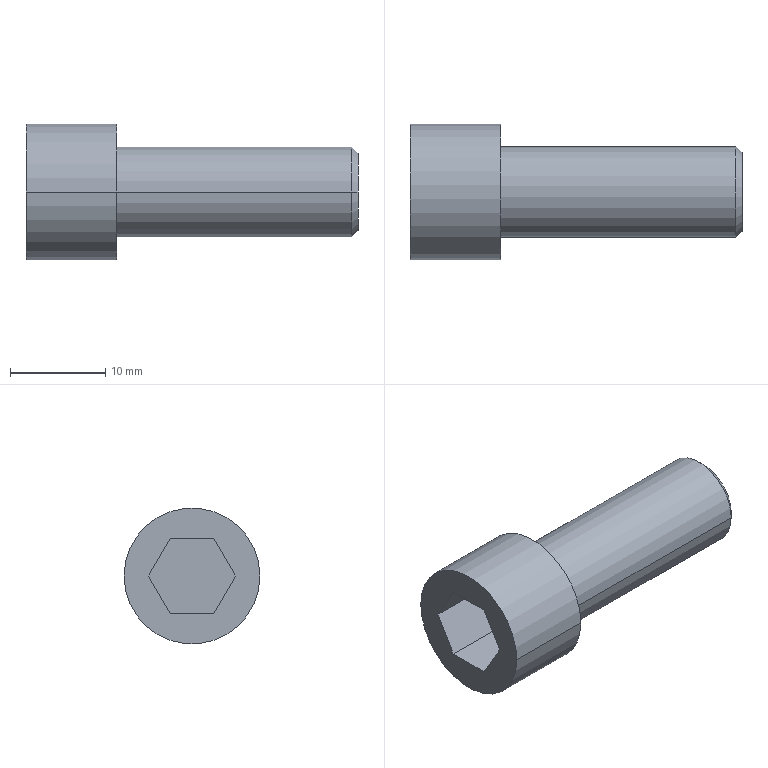Part | STEP file | 4-20.sldasm-Part-69 | 1 solid | 16 faces | box 34.925 x 14.288 x 14.288 mm | volume 2988 mm3 | plane 10 | cylinder 4 | cone 2 | commonest cylinder face diameters 9.525 x2 14.288 x2
STEP:
#1=CARTESIAN_POINT('',(-189.059,-24.456,132.677));
#2=VERTEX_POINT('',#1);
#3=CARTESIAN_POINT('',(-189.059,-32.694,132.677));
#4=VERTEX_POINT('',#3);
#5=CARTESIAN_POINT('',(-189.059,-28.575,132.677));
#6=DIRECTION('',(-1.,0.,0.));
#7=DIRECTION('',(0.,1.,0.));
#8=AXIS2_PLACEMENT_3D('',#5,#6,#7);
#9=CIRCLE('',#8,4.119);
#10=EDGE_CURVE('',#2,#4,#9,.T.);
#11=ORIENTED_EDGE('',*,*,#10,.T.);
#12=CARTESIAN_POINT('',(-189.703,-33.337,132.677));
#13=VERTEX_POINT('',#12);
#14=CARTESIAN_POINT('',(-189.703,-33.337,132.677));
#15=DIRECTION('',(-0.7071,-0.7071,0.));
#16=VECTOR('',#15,1000.);
#17=LINE('',#14,#16);
#18=EDGE_CURVE('',#4,#13,#17,.T.);
#19=ORIENTED_EDGE('',*,*,#18,.T.);
#20=CARTESIAN_POINT('',(-189.703,-23.812,132.677));
#21=VERTEX_POINT('',#20);
#22=CARTESIAN_POINT('',(-189.703,-28.575,132.677));
#23=DIRECTION('',(1.,0.,0.));
#24=DIRECTION('',(0.,1.,0.));
#25=AXIS2_PLACEMENT_3D('',#22,#23,#24);
#26=CIRCLE('',#25,4.762);
#27=EDGE_CURVE('',#13,#21,#26,.T.);
#28=ORIENTED_EDGE('',*,*,#27,.T.);
#29=CARTESIAN_POINT('',(-189.703,-23.812,132.677));
#30=DIRECTION('',(-0.7071,0.7071,0.));
#31=VECTOR('',#30,1000.);
#32=LINE('',#29,#31);
#33=EDGE_CURVE('',#2,#21,#32,.T.);
#34=ORIENTED_EDGE('',*,*,#33,.F.);
#35=EDGE_LOOP('',(#11,#19,#28,#34));
#36=FACE_OUTER_BOUND('',#35,.T.);
#37=CARTESIAN_POINT('',(-189.703,-28.575,132.677));
#38=DIRECTION('',(-1.,0.,0.));
#39=DIRECTION('',(0.,1.,0.));
#40=AXIS2_PLACEMENT_3D('',#37,#38,#39);
#41=CONICAL_SURFACE('',#40,4.762,0.7854);
#42=ADVANCED_FACE('',(#36),#41,.T.);
#43=CARTESIAN_POINT('',(-214.459,-35.719,132.677));
#44=VERTEX_POINT('',#43);
#45=CARTESIAN_POINT('',(-214.459,-21.431,132.677));
#46=VERTEX_POINT('',#45);
#47=CARTESIAN_POINT('',(-214.459,-28.575,132.677));
#48=DIRECTION('',(1.,0.,0.));
#49=DIRECTION('',(0.,1.,0.));
#50=AXIS2_PLACEMENT_3D('',#47,#48,#49);
#51=CIRCLE('',#50,7.144);
#52=EDGE_CURVE('',#44,#46,#51,.T.);
#53=ORIENTED_EDGE('',*,*,#52,.F.);
#54=CARTESIAN_POINT('',(-223.984,-35.719,132.677));
#55=VERTEX_POINT('',#54);
#56=CARTESIAN_POINT('',(-214.459,-35.719,132.677));
#57=DIRECTION('',(-1.,0.,0.));
#58=VECTOR('',#57,1000.);
#59=LINE('',#56,#58);
#60=EDGE_CURVE('',#44,#55,#59,.T.);
#61=ORIENTED_EDGE('',*,*,#60,.T.);
#62=CARTESIAN_POINT('',(-223.984,-21.431,132.677));
#63=VERTEX_POINT('',#62);
#64=CARTESIAN_POINT('',(-223.984,-28.575,132.677));
#65=DIRECTION('',(1.,0.,0.));
#66=DIRECTION('',(0.,1.,0.));
#67=AXIS2_PLACEMENT_3D('',#64,#65,#66);
#68=CIRCLE('',#67,7.144);
#69=EDGE_CURVE('',#55,#63,#68,.T.);
#70=ORIENTED_EDGE('',*,*,#69,.T.);
#71=CARTESIAN_POINT('',(-214.459,-21.431,132.677));
#72=DIRECTION('',(-1.,0.,0.));
#73=VECTOR('',#72,1000.);
#74=LINE('',#71,#73);
#75=EDGE_CURVE('',#46,#63,#74,.T.);
#76=ORIENTED_EDGE('',*,*,#75,.F.);
#77=EDGE_LOOP('',(#53,#61,#70,#76));
#78=FACE_OUTER_BOUND('',#77,.T.);
#79=CARTESIAN_POINT('',(-214.459,-28.575,132.677));
#80=DIRECTION('',(-1.,0.,0.));
#81=DIRECTION('',(0.,1.,0.));
#82=AXIS2_PLACEMENT_3D('',#79,#80,#81);
#83=CYLINDRICAL_SURFACE('',#82,7.144);
#84=ADVANCED_FACE('',(#78),#83,.T.);
#85=CARTESIAN_POINT('',(-214.459,-33.337,132.677));
#86=VERTEX_POINT('',#85);
#87=CARTESIAN_POINT('',(-214.459,-23.812,132.677));
#88=VERTEX_POINT('',#87);
#89=CARTESIAN_POINT('',(-214.459,-28.575,132.677));
#90=DIRECTION('',(1.,0.,0.));
#91=DIRECTION('',(0.,1.,0.));
#92=AXIS2_PLACEMENT_3D('',#89,#90,#91);
#93=CIRCLE('',#92,4.762);
#94=EDGE_CURVE('',#86,#88,#93,.T.);
#95=ORIENTED_EDGE('',*,*,#94,.T.);
#96=CARTESIAN_POINT('',(-214.459,-23.812,132.677));
#97=DIRECTION('',(1.,0.,0.));
#98=VECTOR('',#97,1000.);
#99=LINE('',#96,#98);
#100=EDGE_CURVE('',#88,#21,#99,.T.);
#101=ORIENTED_EDGE('',*,*,#100,.T.);
#102=ORIENTED_EDGE('',*,*,#27,.F.);
#103=CARTESIAN_POINT('',(-214.459,-33.337,132.677));
#104=DIRECTION('',(1.,0.,0.));
#105=VECTOR('',#104,1000.);
#106=LINE('',#103,#105);
#107=EDGE_CURVE('',#86,#13,#106,.T.);
#108=ORIENTED_EDGE('',*,*,#107,.F.);
#109=EDGE_LOOP('',(#95,#101,#102,#108));
#110=FACE_OUTER_BOUND('',#109,.T.);
#111=CARTESIAN_POINT('',(-214.459,-28.575,132.677));
#112=DIRECTION('',(1.,0.,0.));
#113=DIRECTION('',(0.,-1.,0.));
#114=AXIS2_PLACEMENT_3D('',#111,#112,#113);
#115=CYLINDRICAL_SURFACE('',#114,4.763);
#116=ADVANCED_FACE('',(#110),#115,.T.);
#117=ORIENTED_EDGE('',*,*,#100,.F.);
#118=CARTESIAN_POINT('',(-214.459,-28.575,132.677));
#119=DIRECTION('',(1.,0.,0.));
#120=DIRECTION('',(0.,1.,0.));
#121=AXIS2_PLACEMENT_3D('',#118,#119,#120);
#122=CIRCLE('',#121,4.762);
#123=EDGE_CURVE('',#88,#86,#122,.T.);
#124=ORIENTED_EDGE('',*,*,#123,.T.);
#125=ORIENTED_EDGE('',*,*,#107,.T.);
#126=CARTESIAN_POINT('',(-189.703,-28.575,132.677));
#127=DIRECTION('',(1.,0.,0.));
#128=DIRECTION('',(0.,1.,0.));
#129=AXIS2_PLACEMENT_3D('',#126,#127,#128);
#130=CIRCLE('',#129,4.762);
#131=EDGE_CURVE('',#21,#13,#130,.T.);
#132=ORIENTED_EDGE('',*,*,#131,.F.);
#133=EDGE_LOOP('',(#117,#124,#125,#132));
#134=FACE_OUTER_BOUND('',#133,.T.);
#135=CARTESIAN_POINT('',(-214.459,-28.575,132.677));
#136=DIRECTION('',(1.,0.,0.));
#137=DIRECTION('',(0.,-1.,0.));
#138=AXIS2_PLACEMENT_3D('',#135,#136,#137);
#139=CYLINDRICAL_SURFACE('',#138,4.763);
#140=ADVANCED_FACE('',(#134),#139,.T.);
#141=ORIENTED_EDGE('',*,*,#10,.F.);
#142=CARTESIAN_POINT('',(-189.059,-28.575,132.677));
#143=DIRECTION('',(-1.,0.,0.));
#144=DIRECTION('',(0.,1.,0.));
#145=AXIS2_PLACEMENT_3D('',#142,#143,#144);
#146=CIRCLE('',#145,4.119);
#147=EDGE_CURVE('',#4,#2,#146,.T.);
#148=ORIENTED_EDGE('',*,*,#147,.F.);
#149=EDGE_LOOP('',(#141,#148));
#150=FACE_OUTER_BOUND('',#149,.T.);
#151=CARTESIAN_POINT('',(-189.059,-28.575,132.677));
#152=DIRECTION('',(-1.,0.,0.));
#153=DIRECTION('',(0.,1.,0.));
#154=AXIS2_PLACEMENT_3D('',#151,#152,#153);
#155=PLANE('',#154);
#156=ADVANCED_FACE('',(#150),#155,.F.);
#157=CARTESIAN_POINT('',(-214.459,-28.575,132.677));
#158=DIRECTION('',(1.,0.,0.));
#159=DIRECTION('',(0.,1.,0.));
#160=AXIS2_PLACEMENT_3D('',#157,#158,#159);
#161=CIRCLE('',#160,7.144);
#162=EDGE_CURVE('',#46,#44,#161,.T.);
#163=ORIENTED_EDGE('',*,*,#162,.T.);
#164=ORIENTED_EDGE('',*,*,#52,.T.);
#165=EDGE_LOOP('',(#163,#164));
#166=FACE_OUTER_BOUND('',#165,.T.);
#167=ORIENTED_EDGE('',*,*,#94,.F.);
#168=ORIENTED_EDGE('',*,*,#123,.F.);
#169=EDGE_LOOP('',(#167,#168));
#170=FACE_BOUND('',#169,.T.);
#171=CARTESIAN_POINT('',(-214.459,-28.575,132.677));
#172=DIRECTION('',(1.,0.,0.));
#173=DIRECTION('',(0.,-1.,0.));
#174=AXIS2_PLACEMENT_3D('',#171,#172,#173);
#175=PLANE('',#174);
#176=ADVANCED_FACE('',(#166,#170),#175,.T.);
#177=CARTESIAN_POINT('',(-223.984,-30.866,128.708));
#178=VERTEX_POINT('',#177);
#179=CARTESIAN_POINT('',(-223.984,-26.284,128.708));
#180=VERTEX_POINT('',#179);
#181=CARTESIAN_POINT('',(-223.984,-30.866,128.708));
#182=DIRECTION('',(0.,1.,0.));
#183=VECTOR('',#182,1000.);
#184=LINE('',#181,#183);
#185=EDGE_CURVE('',#178,#180,#184,.T.);
#186=ORIENTED_EDGE('',*,*,#185,.T.);
#187=CARTESIAN_POINT('',(-223.984,-23.992,132.677));
#188=VERTEX_POINT('',#187);
#189=CARTESIAN_POINT('',(-223.984,-26.284,128.708));
#190=DIRECTION('',(0.,0.5,0.866));
#191=VECTOR('',#190,1000.);
#192=LINE('',#189,#191);
#193=EDGE_CURVE('',#180,#188,#192,.T.);
#194=ORIENTED_EDGE('',*,*,#193,.T.);
#195=CARTESIAN_POINT('',(-223.984,-26.284,136.646));
#196=VERTEX_POINT('',#195);
#197=CARTESIAN_POINT('',(-223.984,-23.992,132.677));
#198=DIRECTION('',(0.,-0.5,0.866));
#199=VECTOR('',#198,1000.);
#200=LINE('',#197,#199);
#201=EDGE_CURVE('',#188,#196,#200,.T.);
#202=ORIENTED_EDGE('',*,*,#201,.T.);
#203=CARTESIAN_POINT('',(-223.984,-30.866,136.646));
#204=VERTEX_POINT('',#203);
#205=CARTESIAN_POINT('',(-223.984,-26.284,136.646));
#206=DIRECTION('',(0.,-1.,0.));
#207=VECTOR('',#206,1000.);
#208=LINE('',#205,#207);
#209=EDGE_CURVE('',#196,#204,#208,.T.);
#210=ORIENTED_EDGE('',*,*,#209,.T.);
#211=CARTESIAN_POINT('',(-223.984,-33.158,132.677));
#212=VERTEX_POINT('',#211);
#213=CARTESIAN_POINT('',(-223.984,-30.866,136.646));
#214=DIRECTION('',(0.,-0.5,-0.866));
#215=VECTOR('',#214,1000.);
#216=LINE('',#213,#215);
#217=EDGE_CURVE('',#204,#212,#216,.T.);
#218=ORIENTED_EDGE('',*,*,#217,.T.);
#219=CARTESIAN_POINT('',(-223.984,-33.158,132.677));
#220=DIRECTION('',(0.,0.5,-0.866));
#221=VECTOR('',#220,1000.);
#222=LINE('',#219,#221);
#223=EDGE_CURVE('',#212,#178,#222,.T.);
#224=ORIENTED_EDGE('',*,*,#223,.T.);
#225=EDGE_LOOP('',(#186,#194,#202,#210,#218,#224));
#226=FACE_BOUND('',#225,.T.);
#227=CARTESIAN_POINT('',(-223.984,-28.575,132.677));
#228=DIRECTION('',(1.,0.,0.));
#229=DIRECTION('',(0.,1.,0.));
#230=AXIS2_PLACEMENT_3D('',#227,#228,#229);
#231=CIRCLE('',#230,7.144);
#232=EDGE_CURVE('',#63,#55,#231,.T.);
#233=ORIENTED_EDGE('',*,*,#232,.F.);
#234=ORIENTED_EDGE('',*,*,#69,.F.);
#235=EDGE_LOOP('',(#233,#234));
#236=FACE_OUTER_BOUND('',#235,.T.);
#237=CARTESIAN_POINT('',(-223.984,-28.575,132.677));
#238=DIRECTION('',(-1.,0.,0.));
#239=DIRECTION('',(0.,1.,0.));
#240=AXIS2_PLACEMENT_3D('',#237,#238,#239);
#241=PLANE('',#240);
#242=ADVANCED_FACE('',(#226,#236),#241,.T.);
#243=ORIENTED_EDGE('',*,*,#60,.F.);
#244=ORIENTED_EDGE('',*,*,#162,.F.);
#245=ORIENTED_EDGE('',*,*,#75,.T.);
#246=ORIENTED_EDGE('',*,*,#232,.T.);
#247=EDGE_LOOP('',(#243,#244,#245,#246));
#248=FACE_OUTER_BOUND('',#247,.T.);
#249=CARTESIAN_POINT('',(-214.459,-28.575,132.677));
#250=DIRECTION('',(-1.,0.,0.));
#251=DIRECTION('',(0.,1.,0.));
#252=AXIS2_PLACEMENT_3D('',#249,#250,#251);
#253=CYLINDRICAL_SURFACE('',#252,7.144);
#254=ADVANCED_FACE('',(#248),#253,.T.);
#255=ORIENTED_EDGE('',*,*,#18,.F.);
#256=ORIENTED_EDGE('',*,*,#147,.T.);
#257=ORIENTED_EDGE('',*,*,#33,.T.);
#258=ORIENTED_EDGE('',*,*,#131,.T.);
#259=EDGE_LOOP('',(#255,#256,#257,#258));
#260=FACE_OUTER_BOUND('',#259,.T.);
#261=CARTESIAN_POINT('',(-189.703,-28.575,132.677));
#262=DIRECTION('',(-1.,0.,0.));
#263=DIRECTION('',(0.,1.,0.));
#264=AXIS2_PLACEMENT_3D('',#261,#262,#263);
#265=CONICAL_SURFACE('',#264,4.762,0.7854);
#266=ADVANCED_FACE('',(#260),#265,.T.);
#267=ORIENTED_EDGE('',*,*,#185,.F.);
#268=CARTESIAN_POINT('',(-217.697,-30.866,128.708));
#269=VERTEX_POINT('',#268);
#270=CARTESIAN_POINT('',(-217.697,-30.866,128.708));
#271=DIRECTION('',(-1.,0.,0.));
#272=VECTOR('',#271,1000.);
#273=LINE('',#270,#272);
#274=EDGE_CURVE('',#269,#178,#273,.T.);
#275=ORIENTED_EDGE('',*,*,#274,.F.);
#276=CARTESIAN_POINT('',(-217.697,-26.284,128.708));
#277=VERTEX_POINT('',#276);
#278=CARTESIAN_POINT('',(-217.697,-30.866,128.708));
#279=DIRECTION('',(0.,1.,0.));
#280=VECTOR('',#279,1000.);
#281=LINE('',#278,#280);
#282=EDGE_CURVE('',#269,#277,#281,.T.);
#283=ORIENTED_EDGE('',*,*,#282,.T.);
#284=CARTESIAN_POINT('',(-217.697,-26.284,128.708));
#285=DIRECTION('',(-1.,0.,0.));
#286=VECTOR('',#285,1000.);
#287=LINE('',#284,#286);
#288=EDGE_CURVE('',#277,#180,#287,.T.);
#289=ORIENTED_EDGE('',*,*,#288,.T.);
#290=EDGE_LOOP('',(#267,#275,#283,#289));
#291=FACE_OUTER_BOUND('',#290,.T.);
#292=CARTESIAN_POINT('',(-217.697,-30.866,128.708));
#293=DIRECTION('',(0.,0.,-1.));
#294=DIRECTION('',(1.,0.,0.));
#295=AXIS2_PLACEMENT_3D('',#292,#293,#294);
#296=PLANE('',#295);
#297=ADVANCED_FACE('',(#291),#296,.F.);
#298=ORIENTED_EDGE('',*,*,#193,.F.);
#299=ORIENTED_EDGE('',*,*,#288,.F.);
#300=CARTESIAN_POINT('',(-217.697,-23.992,132.677));
#301=VERTEX_POINT('',#300);
#302=CARTESIAN_POINT('',(-217.697,-26.284,128.708));
#303=DIRECTION('',(0.,0.5,0.866));
#304=VECTOR('',#303,1000.);
#305=LINE('',#302,#304);
#306=EDGE_CURVE('',#277,#301,#305,.T.);
#307=ORIENTED_EDGE('',*,*,#306,.T.);
#308=CARTESIAN_POINT('',(-217.697,-23.992,132.677));
#309=DIRECTION('',(-1.,0.,0.));
#310=VECTOR('',#309,1000.);
#311=LINE('',#308,#310);
#312=EDGE_CURVE('',#301,#188,#311,.T.);
#313=ORIENTED_EDGE('',*,*,#312,.T.);
#314=EDGE_LOOP('',(#298,#299,#307,#313));
#315=FACE_OUTER_BOUND('',#314,.T.);
#316=CARTESIAN_POINT('',(-217.697,-26.284,128.708));
#317=DIRECTION('',(0.,0.866,-0.5));
#318=DIRECTION('',(0.,0.5,0.866));
#319=AXIS2_PLACEMENT_3D('',#316,#317,#318);
#320=PLANE('',#319);
#321=ADVANCED_FACE('',(#315),#320,.F.);
#322=ORIENTED_EDGE('',*,*,#201,.F.);
#323=ORIENTED_EDGE('',*,*,#312,.F.);
#324=CARTESIAN_POINT('',(-217.697,-26.284,136.646));
#325=VERTEX_POINT('',#324);
#326=CARTESIAN_POINT('',(-217.697,-23.992,132.677));
#327=DIRECTION('',(0.,-0.5,0.866));
#328=VECTOR('',#327,1000.);
#329=LINE('',#326,#328);
#330=EDGE_CURVE('',#301,#325,#329,.T.);
#331=ORIENTED_EDGE('',*,*,#330,.T.);
#332=CARTESIAN_POINT('',(-217.697,-26.284,136.646));
#333=DIRECTION('',(-1.,0.,0.));
#334=VECTOR('',#333,1000.);
#335=LINE('',#332,#334);
#336=EDGE_CURVE('',#325,#196,#335,.T.);
#337=ORIENTED_EDGE('',*,*,#336,.T.);
#338=EDGE_LOOP('',(#322,#323,#331,#337));
#339=FACE_OUTER_BOUND('',#338,.T.);
#340=CARTESIAN_POINT('',(-217.697,-23.992,132.677));
#341=DIRECTION('',(0.,0.866,0.5));
#342=DIRECTION('',(0.,-0.5,0.866));
#343=AXIS2_PLACEMENT_3D('',#340,#341,#342);
#344=PLANE('',#343);
#345=ADVANCED_FACE('',(#339),#344,.F.);
#346=ORIENTED_EDGE('',*,*,#209,.F.);
#347=ORIENTED_EDGE('',*,*,#336,.F.);
#348=CARTESIAN_POINT('',(-217.697,-30.866,136.646));
#349=VERTEX_POINT('',#348);
#350=CARTESIAN_POINT('',(-217.697,-26.284,136.646));
#351=DIRECTION('',(0.,-1.,0.));
#352=VECTOR('',#351,1000.);
#353=LINE('',#350,#352);
#354=EDGE_CURVE('',#325,#349,#353,.T.);
#355=ORIENTED_EDGE('',*,*,#354,.T.);
#356=CARTESIAN_POINT('',(-217.697,-30.866,136.646));
#357=DIRECTION('',(-1.,0.,0.));
#358=VECTOR('',#357,1000.);
#359=LINE('',#356,#358);
#360=EDGE_CURVE('',#349,#204,#359,.T.);
#361=ORIENTED_EDGE('',*,*,#360,.T.);
#362=EDGE_LOOP('',(#346,#347,#355,#361));
#363=FACE_OUTER_BOUND('',#362,.T.);
#364=CARTESIAN_POINT('',(-217.697,-26.284,136.646));
#365=DIRECTION('',(0.,0.,1.));
#366=DIRECTION('',(-1.,0.,0.));
#367=AXIS2_PLACEMENT_3D('',#364,#365,#366);
#368=PLANE('',#367);
#369=ADVANCED_FACE('',(#363),#368,.F.);
#370=ORIENTED_EDGE('',*,*,#217,.F.);
#371=ORIENTED_EDGE('',*,*,#360,.F.);
#372=CARTESIAN_POINT('',(-217.697,-33.158,132.677));
#373=VERTEX_POINT('',#372);
#374=CARTESIAN_POINT('',(-217.697,-30.866,136.646));
#375=DIRECTION('',(0.,-0.5,-0.866));
#376=VECTOR('',#375,1000.);
#377=LINE('',#374,#376);
#378=EDGE_CURVE('',#349,#373,#377,.T.);
#379=ORIENTED_EDGE('',*,*,#378,.T.);
#380=CARTESIAN_POINT('',(-217.697,-33.158,132.677));
#381=DIRECTION('',(-1.,0.,0.));
#382=VECTOR('',#381,1000.);
#383=LINE('',#380,#382);
#384=EDGE_CURVE('',#373,#212,#383,.T.);
#385=ORIENTED_EDGE('',*,*,#384,.T.);
#386=EDGE_LOOP('',(#370,#371,#379,#385));
#387=FACE_OUTER_BOUND('',#386,.T.);
#388=CARTESIAN_POINT('',(-217.697,-30.866,136.646));
#389=DIRECTION('',(0.,-0.866,0.5));
#390=DIRECTION('',(0.,-0.5,-0.866));
#391=AXIS2_PLACEMENT_3D('',#388,#389,#390);
#392=PLANE('',#391);
#393=ADVANCED_FACE('',(#387),#392,.F.);
#394=ORIENTED_EDGE('',*,*,#223,.F.);
#395=ORIENTED_EDGE('',*,*,#384,.F.);
#396=CARTESIAN_POINT('',(-217.697,-33.158,132.677));
#397=DIRECTION('',(0.,0.5,-0.866));
#398=VECTOR('',#397,1000.);
#399=LINE('',#396,#398);
#400=EDGE_CURVE('',#373,#269,#399,.T.);
#401=ORIENTED_EDGE('',*,*,#400,.T.);
#402=ORIENTED_EDGE('',*,*,#274,.T.);
#403=EDGE_LOOP('',(#394,#395,#401,#402));
#404=FACE_OUTER_BOUND('',#403,.T.);
#405=CARTESIAN_POINT('',(-217.697,-33.158,132.677));
#406=DIRECTION('',(0.,-0.866,-0.5));
#407=DIRECTION('',(0.,0.5,-0.866));
#408=AXIS2_PLACEMENT_3D('',#405,#406,#407);
#409=PLANE('',#408);
#410=ADVANCED_FACE('',(#404),#409,.F.);
#411=ORIENTED_EDGE('',*,*,#282,.F.);
#412=ORIENTED_EDGE('',*,*,#400,.F.);
#413=ORIENTED_EDGE('',*,*,#378,.F.);
#414=ORIENTED_EDGE('',*,*,#354,.F.);
#415=ORIENTED_EDGE('',*,*,#330,.F.);
#416=ORIENTED_EDGE('',*,*,#306,.F.);
#417=EDGE_LOOP('',(#411,#412,#413,#414,#415,#416));
#418=FACE_OUTER_BOUND('',#417,.T.);
#419=CARTESIAN_POINT('',(-217.697,-26.284,128.708));
#420=DIRECTION('',(-1.,0.,0.));
#421=DIRECTION('',(0.,1.,0.));
#422=AXIS2_PLACEMENT_3D('',#419,#420,#421);
#423=PLANE('',#422);
#424=ADVANCED_FACE('',(#418),#423,.T.);
#425=CLOSED_SHELL('',(#42,#84,#116,#140,#156,#176,#242,#254,#266,#297,#321,#345,#369,#393,#410,#424));
#426=MANIFOLD_SOLID_BREP('',#425);
#427=CARTESIAN_POINT('',(0.,0.,0.));
#428=DIRECTION('',(0.,0.,1.));
#429=DIRECTION('',(1.,0.,0.));
#430=AXIS2_PLACEMENT_3D('',#427,#428,#429);
#431=(LENGTH_UNIT()NAMED_UNIT(*)SI_UNIT(.MILLI.,.METRE.));
#432=UNCERTAINTY_MEASURE_WITH_UNIT(LENGTH_MEASURE(0.00001),#431,'','');
#433=(NAMED_UNIT(*)PLANE_ANGLE_UNIT()SI_UNIT($,.RADIAN.));
#434=(NAMED_UNIT(*)SI_UNIT($,.STERADIAN.)SOLID_ANGLE_UNIT());
#435=(GEOMETRIC_REPRESENTATION_CONTEXT(3)GLOBAL_UNCERTAINTY_ASSIGNED_CONTEXT((#432))GLOBAL_UNIT_ASSIGNED_CONTEXT((#431,#433,#434))REPRESENTATION_CONTEXT('',''));
#436=ADVANCED_BREP_SHAPE_REPRESENTATION('',(#426,#430),#435);